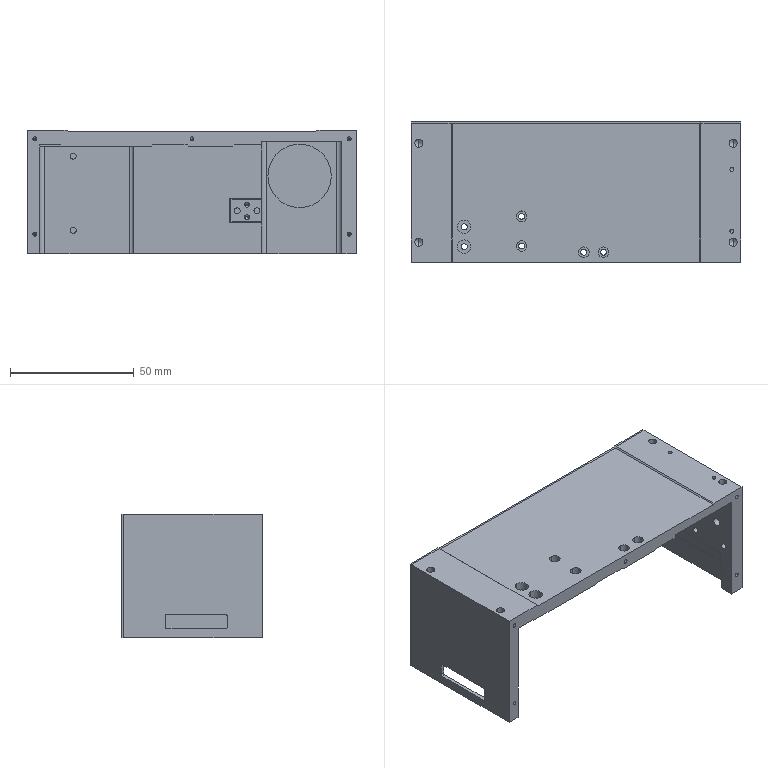NC program | NX | posted with a generic post | part box 133 x 56.74 x 50 mm
Lines 302 to 1465 of 22463:
(CAVITY_MILL , TOOL : D10)
N584 T10 M6
N586 G54
N588 G17 G0 G90 X4.555 Y-36.169 B0. C0. S9500 M3
N590 G43 Z30. H10
N592 Z1.005
N594 G94 G1 Z-0.495 F1000.
N596 X0.513 Y-29.169
N598 G3 X-0.353 Y-28.669 R1.
N600 G1 Y-7.669
N602 X37.695 F3000.
N604 G2 X38.9 Y-5.314 R26.1
N606 G1 Y-3.47
N608 X30.655
N610 G2 X23.5 Y-4.47 R26.1
N612 G1 X-28.25
N614 G2 X-38.4 Y-2.416 R26.1
N616 G1 Y-7.669
N618 X-0.353
N620 Y-14.669
N622 X42.762
N624 G2 X45.9 Y-7.35 R19.1
N626 G1 Y3.53
N628 X29.599
N630 G2 X23.5 Y2.53 R19.1
N632 G1 X-28.25
N634 G2 X-38.526 Y5.53 R19.1
N636 G1 X-45.4
N638 Y-10.674
N640 G2 X-43.021 Y-14.669 R19.1
N642 G1 X-0.353
N644 Y-21.669
N646 X49.4
N648 Y-18.37
N650 G2 X52.9 Y-9.858 R12.1
N652 G1 Y10.53
N654 X28.317
N656 G2 X23.5 Y9.53 R12.1
N658 G1 X-28.25
N660 G2 X-36.225 Y12.53 R12.1
N662 G1 X-49.527
N664 G2 X-52.4 Y8.641 R12.1
N666 G1 Y-13.381
N668 G2 X-48.42 Y-21.669 R12.1
N670 G1 X-0.353
N672 Y-28.669
N674 X55.007
N676 G3 X55.1 Y-29.506 R6.5
N678 G1 Y-33.169
N680 X56.5
N682 Y-29.375
N684 G2 X56.4 Y-28.37 R5.1
N686 G1 Y-18.37
N688 G2 X59.9 Y-13.527 R5.1
N690 G1 Y14.787
N692 G2 X56.852 Y17.53 R5.1
N694 G1 X26.533
N696 G2 X23.5 Y16.53 R5.1
N698 G1 X-28.25
N700 G2 X-32.898 Y19.53 R5.1
N702 G1 X-55.4
N704 Y17.395
N706 X-55.405 Y17.396
N708 G2 X-59.4 Y12.65 R5.1
N710 G1 Y-17.39
N712 G2 X-55.4 Y-22.37 R5.1
N714 G1 Y-28.37
N716 G2 X-55.5 Y-29.375 R5.1
N718 G1 Y-33.169
N720 X-54.1
N722 Y-29.506
N724 G3 X-54.007 Y-28.669 R6.5
N726 G1 X-0.353
N728 G2 X0.513 Y-29.169 R1.
N730 G1 X4.555 Y-36.169
N732 Z1.005
N734 G0 Z0.511
N736 G1 Z-0.989 F1000.
N738 X0.513 Y-29.169
N740 G3 X-0.353 Y-28.669 R1.
N742 G1 Y-7.669
N744 X37.695 F3000.
N746 G2 X38.9 Y-5.314 R26.1
N748 G1 Y-3.47
N750 X30.655
N752 G2 X23.5 Y-4.47 R26.1
N754 G1 X-28.25
N756 G2 X-38.4 Y-2.416 R26.1
N758 G1 Y-7.669
N760 X-0.353
N762 Y-14.669
N764 X42.762
N766 G2 X45.9 Y-7.35 R19.1
N768 G1 Y3.53
N770 X29.599
N772 G2 X23.5 Y2.53 R19.1
N774 G1 X-28.25
N776 G2 X-38.526 Y5.53 R19.1
N778 G1 X-45.4
N780 Y-10.674
N782 G2 X-43.021 Y-14.669 R19.1
N784 G1 X-0.353
N786 Y-21.669
N788 X49.4
N790 Y-18.369
N792 G2 X52.9 Y-9.858 R12.1
N794 G1 Y10.53
N796 X28.317
N798 G2 X23.5 Y9.53 R12.1
N800 G1 X-28.25
N802 G2 X-36.225 Y12.53 R12.1
N804 G1 X-49.527
N806 G2 X-52.4 Y8.641 R12.1
N808 G1 Y-13.381
N810 G2 X-48.42 Y-21.669 R12.1
N812 G1 X-0.353
N814 Y-28.669
N816 X55.007
N818 G3 X55.1 Y-29.506 R6.5
N820 G1 Y-33.169
N822 X56.5
N824 Y-29.375
N826 G2 X56.4 Y-28.37 R5.1
N828 G1 Y-21.669
N830 Y-18.369
N832 G2 X59.9 Y-13.527 R5.1
N834 G1 Y14.787
N836 G2 X56.852 Y17.53 R5.1
N838 G1 X26.533
N840 G2 X23.5 Y16.53 R5.1
N842 G1 X-28.25
N844 G2 X-32.898 Y19.53 R5.1
N846 G1 X-55.4
N848 Y17.395
N850 X-55.405 Y17.396
N852 G2 X-59.4 Y12.65 R5.1
N854 G1 Y-17.39
N856 G2 X-55.4 Y-22.37 R5.1
N858 G1 Y-28.37
N860 G2 X-55.5 Y-29.375 R5.1
N862 G1 Y-33.169
N864 X-54.1
N866 Y-29.506
N868 G3 X-54.007 Y-28.669 R6.5
N870 G1 X-0.353
N872 G2 X0.513 Y-29.169 R1.
N874 G1 X4.555 Y-36.169
N876 Z0.511
N878 G0 Z0.016
N880 G1 Z-1.484 F1000.
N882 X0.513 Y-29.169
N884 G3 X-0.353 Y-28.669 R1.
N886 G1 Y-7.669
N888 X37.695 F3000.
N890 G2 X38.9 Y-5.314 R26.1
N892 G1 Y-3.47
N894 X30.655
N896 G2 X23.5 Y-4.47 R26.1
N898 G1 X-28.25
N900 G2 X-38.4 Y-2.416 R26.1
N902 G1 Y-7.669
N904 X-0.353
N906 Y-14.669
N908 X42.762
N910 G2 X45.9 Y-7.35 R19.1
N912 G1 Y3.53
N914 X29.599
N916 G2 X23.5 Y2.53 R19.1
N918 G1 X-28.25
N920 G2 X-38.526 Y5.53 R19.1
N922 G1 X-45.4
N924 Y-10.674
N926 G2 X-43.021 Y-14.669 R19.1
N928 G1 X-0.353
N930 Y-21.669
N932 X49.4
N934 Y-18.37
N936 G2 X52.9 Y-9.858 R12.1
N938 G1 Y10.53
N940 X28.317
N942 G2 X23.5 Y9.53 R12.1
N944 G1 X-28.25
N946 G2 X-36.225 Y12.53 R12.1
N948 G1 X-49.527
N950 G2 X-52.4 Y8.641 R12.1
N952 G1 Y-13.381
N954 G2 X-48.42 Y-21.669 R12.1
N956 G1 X-0.353
N958 Y-28.669
N960 X55.007
N962 G3 X55.1 Y-29.506 R6.5
N964 G1 Y-33.169
N966 X56.5
N968 Y-29.375
N970 G2 X56.4 Y-28.37 R5.1
N972 G1 Y-18.37
N974 G2 X59.9 Y-13.527 R5.1
N976 G1 Y14.787
N978 G2 X56.852 Y17.53 R5.1
N980 G1 X26.533
N982 G2 X23.5 Y16.53 R5.1
N984 G1 X-28.25
N986 G2 X-32.898 Y19.53 R5.1
N988 G1 X-55.4
N990 Y17.395
N992 X-55.405 Y17.396
N994 G2 X-59.4 Y12.65 R5.1
N996 G1 Y-17.39
N998 G2 X-55.4 Y-22.37 R5.1
N1000 G1 Y-28.37
N1002 G2 X-55.5 Y-29.375 R5.1
N1004 G1 Y-33.169
N1006 X-54.1
N1008 Y-29.506
N1010 G3 X-54.007 Y-28.669 R6.5
N1012 G1 X-0.353
N1014 G2 X0.513 Y-29.169 R1.
N1016 G1 X4.555 Y-36.169
N1018 Z0.016
N1020 G0 Z-0.479
N1022 G1 Z-1.979 F1000.
N1024 X0.513 Y-29.169
N1026 G3 X-0.353 Y-28.669 R1.
N1028 G1 Y-7.669
N1030 X37.695 F3000.
N1032 G2 X38.9 Y-5.314 R26.1
N1034 G1 Y-3.47
N1036 X30.655
N1038 G2 X23.5 Y-4.47 R26.1
N1040 G1 X-28.25
N1042 G2 X-38.4 Y-2.416 R26.1
N1044 G1 Y-7.669
N1046 X-0.353
N1048 Y-14.669
N1050 X42.762
N1052 G2 X45.9 Y-7.35 R19.1
N1054 G1 Y3.53
N1056 X29.599
N1058 G2 X23.5 Y2.53 R19.1
N1060 G1 X-28.25
N1062 G2 X-38.526 Y5.53 R19.1
N1064 G1 X-45.4
N1066 Y-10.674
N1068 G2 X-43.021 Y-14.669 R19.1
N1070 G1 X-0.353
N1072 Y-21.669
N1074 X49.4
N1076 Y-18.37
N1078 G2 X52.9 Y-9.858 R12.1
N1080 G1 Y10.53
N1082 X28.317
N1084 G2 X23.5 Y9.53 R12.1
N1086 G1 X-28.25
N1088 G2 X-36.225 Y12.53 R12.1
N1090 G1 X-49.527
N1092 G2 X-52.4 Y8.641 R12.1
N1094 G1 Y-13.381
N1096 G2 X-48.42 Y-21.669 R12.1
N1098 G1 X-0.353
N1100 Y-28.669
N1102 X55.007
N1104 G3 X55.1 Y-29.506 R6.5
N1106 G1 Y-33.169
N1108 X56.5
N1110 Y-29.375
N1112 G2 X56.4 Y-28.37 R5.1
N1114 G1 Y-18.37
N1116 G2 X59.9 Y-13.527 R5.1
N1118 G1 Y14.787
N1120 G2 X56.852 Y17.53 R5.1
N1122 G1 X26.533
N1124 G2 X23.5 Y16.53 R5.1
N1126 G1 X-28.25
N1128 G2 X-32.898 Y19.53 R5.1
N1130 G1 X-55.4
N1132 Y17.395
N1134 X-55.405 Y17.396
N1136 G2 X-59.4 Y12.65 R5.1
N1138 G1 Y-17.39
N1140 G2 X-55.4 Y-22.37 R5.1
N1142 G1 Y-28.37
N1144 G2 X-55.5 Y-29.375 R5.1
N1146 G1 Y-33.169
N1148 X-54.1
N1150 Y-29.506
N1152 G3 X-54.007 Y-28.669 R6.5
N1154 G1 X-0.353
N1156 G2 X0.513 Y-29.169 R1.
N1158 G1 X4.555 Y-36.169
N1160 Z-0.479
N1162 G0 Z-0.974
N1164 G1 Z-2.474 F1000.
N1166 X0.513 Y-29.169
N1168 G3 X-0.353 Y-28.669 R1.
N1170 G1 Y-7.669
N1172 X37.695 F3000.
N1174 G2 X38.9 Y-5.314 R26.1
N1176 G1 Y-3.47
N1178 X30.655
N1180 G2 X23.5 Y-4.47 R26.1
N1182 G1 X-28.25
N1184 G2 X-38.4 Y-2.416 R26.1
N1186 G1 Y-7.669
N1188 X-0.353
N1190 Y-14.669
N1192 X42.762
N1194 G2 X45.9 Y-7.35 R19.1
N1196 G1 Y3.53
N1198 X29.599
N1200 G2 X23.5 Y2.53 R19.1
N1202 G1 X-28.25
N1204 G2 X-38.526 Y5.53 R19.1
N1206 G1 X-45.4
N1208 Y-10.674
N1210 G2 X-43.021 Y-14.669 R19.1
N1212 G1 X-0.353
N1214 Y-21.669
N1216 X49.4
N1218 Y-18.37
N1220 G2 X52.9 Y-9.858 R12.1
N1222 G1 Y10.53
N1224 X28.317
N1226 G2 X23.5 Y9.53 R12.1
N1228 G1 X-28.25
N1230 G2 X-36.225 Y12.53 R12.1
N1232 G1 X-49.527
N1234 G2 X-52.4 Y8.641 R12.1
N1236 G1 Y-13.381
N1238 G2 X-48.42 Y-21.669 R12.1
N1240 G1 X-0.353
N1242 Y-28.669
N1244 X55.007
N1246 G3 X55.1 Y-29.506 R6.5
N1248 G1 Y-33.169
N1250 X56.5
N1252 Y-29.375
N1254 G2 X56.4 Y-28.37 R5.1
N1256 G1 Y-18.37
N1258 G2 X59.9 Y-13.527 R5.1
N1260 G1 Y14.787
N1262 G2 X56.852 Y17.53 R5.1
N1264 G1 X26.533
N1266 G2 X23.5 Y16.53 R5.1
N1268 G1 X-28.25
N1270 G2 X-32.898 Y19.53 R5.1
N1272 G1 X-55.4
N1274 Y17.395
N1276 X-55.405 Y17.396
N1278 G2 X-59.4 Y12.65 R5.1
N1280 G1 Y-17.39
N1282 G2 X-55.4 Y-22.37 R5.1
N1284 G1 Y-28.37
N1286 G2 X-55.5 Y-29.375 R5.1
N1288 G1 Y-33.169
N1290 X-54.1
N1292 Y-29.506
N1294 G3 X-54.007 Y-28.669 R6.5
N1296 G1 X-0.353
N1298 G2 X0.513 Y-29.169 R1.
N1300 G1 X4.555 Y-36.169
N1302 Z-0.974
N1304 G0 Z-1.468
N1306 G1 Z-2.968 F1000.
N1308 X0.513 Y-29.169
N1310 G3 X-0.353 Y-28.669 R1.
N1312 G1 Y-7.669
N1314 X37.695 F3000.
N1316 G2 X38.9 Y-5.314 R26.1
N1318 G1 Y-3.47
N1320 X30.655
N1322 G2 X23.5 Y-4.47 R26.1
N1324 G1 X-28.25
N1326 G2 X-38.4 Y-2.416 R26.1
N1328 G1 Y-7.669
N1330 X-0.353
N1332 Y-14.669
N1334 X42.762
N1336 G2 X45.9 Y-7.35 R19.1
N1338 G1 Y3.53
N1340 X29.599
N1342 G2 X23.5 Y2.53 R19.1
N1344 G1 X-28.25
N1346 G2 X-38.526 Y5.53 R19.1
N1348 G1 X-45.4
N1350 Y-10.674
N1352 G2 X-43.021 Y-14.669 R19.1
N1354 G1 X-0.353
N1356 Y-21.669
N1358 X49.4
N1360 Y-18.37
N1362 G2 X52.9 Y-9.858 R12.1
N1364 G1 Y10.53
N1366 X28.317
N1368 G2 X23.5 Y9.53 R12.1
N1370 G1 X-28.25
N1372 G2 X-36.225 Y12.53 R12.1
N1374 G1 X-49.527
N1376 G2 X-52.4 Y8.641 R12.1
N1378 G1 Y-13.381
N1380 G2 X-48.42 Y-21.669 R12.1
N1382 G1 X-0.353
N1384 Y-28.669
N1386 X55.007
N1388 G3 X55.1 Y-29.506 R6.5
N1390 G1 Y-33.169
N1392 X56.5
N1394 Y-29.375
N1396 G2 X56.4 Y-28.37 R5.1
N1398 G1 Y-18.37
N1400 G2 X59.9 Y-13.527 R5.1
N1402 G1 Y14.787
N1404 G2 X56.852 Y17.53 R5.1
N1406 G1 X26.533
N1408 G2 X23.5 Y16.53 R5.1
N1410 G1 X-28.25
N1412 G2 X-32.898 Y19.53 R5.1
N1414 G1 X-55.4
N1416 Y17.395
N1418 X-55.405 Y17.396
N1420 G2 X-59.4 Y12.65 R5.1
N1422 G1 Y-17.39
N1424 G2 X-55.4 Y-22.37 R5.1
N1426 G1 Y-28.37
N1428 G2 X-55.5 Y-29.375 R5.1
N1430 G1 Y-33.169
N1432 X-54.1
N1434 Y-29.506
N1436 G3 X-54.007 Y-28.669 R6.5
N1438 G1 X-0.353
N1440 G2 X0.513 Y-29.169 R1.
N1442 G1 X4.555 Y-36.169
N1444 Z-1.468
N1446 G0 Z-1.963
N1448 G1 Z-3.463 F1000.
N1450 X0.513 Y-29.169
N1452 G3 X-0.353 Y-28.669 R1.
N1454 G1 Y-7.669
N1456 X37.695 F3000.
N1458 G2 X38.9 Y-5.314 R26.1
N1460 G1 Y-3.47
N1462 X30.655
N1464 G2 X23.5 Y-4.47 R26.1
N1466 G1 X-28.25
N1468 G2 X-38.4 Y-2.416 R26.1
N1470 G1 Y-7.669
N1472 X-0.353
N1474 Y-14.669
N1476 X42.762
N1478 G2 X45.9 Y-7.35 R19.1
N1480 G1 Y3.53
N1482 X29.599
N1484 G2 X23.5 Y2.53 R19.1
N1486 G1 X-28.25
N1488 G2 X-38.526 Y5.53 R19.1
N1490 G1 X-45.4
N1492 Y-10.674
N1494 G2 X-43.021 Y-14.669 R19.1
N1496 G1 X-0.353
N1498 Y-21.669
N1500 X49.4
N1502 Y-18.37
N1504 G2 X52.9 Y-9.858 R12.1
N1506 G1 Y10.53
N1508 X28.317
N1510 G2 X23.5 Y9.53 R12.1
N1512 G1 X-28.25
N1514 G2 X-36.225 Y12.53 R12.1
N1516 G1 X-49.527
N1518 G2 X-52.4 Y8.641 R12.1
N1520 G1 Y-13.381
N1522 G2 X-48.42 Y-21.669 R12.1
N1524 G1 X-0.353
N1526 Y-28.669
N1528 X55.007
N1530 G3 X55.1 Y-29.506 R6.5
N1532 G1 Y-33.169
N1534 X56.5
N1536 Y-29.375
N1538 G2 X56.4 Y-28.37 R5.1
N1540 G1 Y-18.37
N1542 G2 X59.9 Y-13.527 R5.1
N1544 G1 Y14.787
N1546 G2 X56.852 Y17.53 R5.1
N1548 G1 X26.533
N1550 G2 X23.5 Y16.53 R5.1
N1552 G1 X-28.25
N1554 G2 X-32.898 Y19.53 R5.1
N1556 G1 X-55.4
N1558 Y17.395
N1560 X-55.405 Y17.396
N1562 G2 X-59.4 Y12.65 R5.1
N1564 G1 Y-17.39
N1566 G2 X-55.4 Y-22.37 R5.1
N1568 G1 Y-28.37
N1570 G2 X-55.5 Y-29.375 R5.1
N1572 G1 Y-33.169
N1574 X-54.1
N1576 Y-29.506
N1578 G3 X-54.007 Y-28.669 R6.5
N1580 G1 X-0.353
N1582 G2 X0.513 Y-29.169 R1.
N1584 G1 X4.555 Y-36.169
N1586 Z-1.963
N1588 G0 Z-2.458
N1590 G1 Z-3.958 F1000.
N1592 X0.513 Y-29.169
N1594 G3 X-0.353 Y-28.669 R1.
N1596 G1 Y-7.669
N1598 X37.695 F3000.
N1600 G2 X38.9 Y-5.314 R26.1
N1602 G1 Y-3.47
N1604 X30.655
N1606 G2 X23.5 Y-4.47 R26.1
N1608 G1 X-28.25
N1610 G2 X-38.4 Y-2.416 R26.1
N1612 G1 Y-7.669
N1614 X-0.353
N1616 Y-14.669
N1618 X42.762
N1620 G2 X45.9 Y-7.35 R19.1
N1622 G1 Y3.53
N1624 X29.599
N1626 G2 X23.5 Y2.53 R19.1
N1628 G1 X-28.25
N1630 G2 X-38.526 Y5.53 R19.1
N1632 G1 X-45.4
N1634 Y-10.674
N1636 G2 X-43.021 Y-14.669 R19.1
N1638 G1 X-0.353
N1640 Y-21.669
N1642 X49.4
N1644 Y-18.37
N1646 G2 X52.9 Y-9.858 R12.1
N1648 G1 Y10.53
N1650 X28.317
N1652 G2 X23.5 Y9.53 R12.1
N1654 G1 X-28.25
N1656 G2 X-36.225 Y12.53 R12.1
N1658 G1 X-49.527
N1660 G2 X-52.4 Y8.641 R12.1
N1662 G1 Y-13.381
N1664 G2 X-48.42 Y-21.669 R12.1
N1666 G1 X-0.353
N1668 Y-28.669
N1670 X55.007
N1672 G3 X55.1 Y-29.506 R6.5
N1674 G1 Y-33.169
N1676 X56.5
N1678 Y-29.375
N1680 G2 X56.4 Y-28.37 R5.1
N1682 G1 Y-18.37
N1684 G2 X59.9 Y-13.527 R5.1
N1686 G1 Y14.787
N1688 G2 X56.852 Y17.53 R5.1
N1690 G1 X26.533
N1692 G2 X23.5 Y16.53 R5.1
N1694 G1 X-28.25
N1696 G2 X-32.898 Y19.53 R5.1
N1698 G1 X-55.4
N1700 Y17.395
N1702 X-55.405 Y17.396
N1704 G2 X-59.4 Y12.65 R5.1
N1706 G1 Y-17.39
N1708 G2 X-55.4 Y-22.37 R5.1
N1710 G1 Y-28.37
N1712 G2 X-55.5 Y-29.375 R5.1
N1714 G1 Y-33.169
N1716 X-54.1
N1718 Y-29.506
N1720 G3 X-54.007 Y-28.669 R6.5
N1722 G1 X-0.353
N1724 G2 X0.513 Y-29.169 R1.
N1726 G1 X4.555 Y-36.169
N1728 Z-2.458
N1730 G0 Z-2.953
N1732 G1 Z-4.453 F1000.
N1734 X0.513 Y-29.169
N1736 G3 X-0.353 Y-28.669 R1.
N1738 G1 Y-7.669
N1740 X37.695 F3000.
N1742 G2 X38.9 Y-5.314 R26.1
N1744 G1 Y-3.47
N1746 X30.655
N1748 G2 X23.5 Y-4.47 R26.1
N1750 G1 X-28.25
N1752 G2 X-38.4 Y-2.416 R26.1
N1754 G1 Y-7.669
N1756 X-0.353
N1758 Y-14.669
N1760 X42.762
N1762 G2 X45.9 Y-7.35 R19.1
N1764 G1 Y3.53
N1766 X29.599
N1768 G2 X23.5 Y2.53 R19.1
N1770 G1 X-28.25
N1772 G2 X-38.526 Y5.53 R19.1
N1774 G1 X-45.4
N1776 Y-10.674
N1778 G2 X-43.021 Y-14.669 R19.1
N1780 G1 X-0.353
N1782 Y-21.669
N1784 X49.4
N1786 Y-18.37
N1788 G2 X52.9 Y-9.858 R12.1
N1790 G1 Y10.53
N1792 X28.317
N1794 G2 X23.5 Y9.53 R12.1
N1796 G1 X-28.25
N1798 G2 X-36.225 Y12.53 R12.1
N1800 G1 X-49.527
N1802 G2 X-52.4 Y8.641 R12.1
N1804 G1 Y-13.381
N1806 G2 X-48.42 Y-21.669 R12.1
N1808 G1 X-0.353
N1810 Y-28.669
N1812 X55.007
N1814 G3 X55.1 Y-29.506 R6.5
N1816 G1 Y-33.169
N1818 X56.5
N1820 Y-29.375
N1822 G2 X56.4 Y-28.37 R5.1
N1824 G1 Y-18.37
N1826 G2 X59.9 Y-13.527 R5.1
N1828 G1 Y14.787
N1830 G2 X56.852 Y17.53 R5.1
N1832 G1 X26.533
N1834 G2 X23.5 Y16.53 R5.1
N1836 G1 X-28.25
N1838 G2 X-32.898 Y19.53 R5.1
N1840 G1 X-55.4
N1842 X-55.405 Y17.396
N1844 G2 X-59.4 Y12.65 R5.1
N1846 G1 Y-17.39
N1848 G2 X-55.4 Y-22.37 R5.1
N1850 G1 Y-28.37
N1852 G2 X-55.5 Y-29.375 R5.1
N1854 G1 Y-33.169
N1856 X-54.1
N1858 Y-29.506
N1860 G3 X-54.007 Y-28.669 R6.5
N1862 G1 X-0.353
N1864 G2 X0.513 Y-29.169 R1.
N1866 G1 X4.555 Y-36.169
N1868 Z-2.953
N1870 G0 Z-3.447
N1872 G1 Z-4.947 F1000.
N1874 X0.513 Y-29.169
N1876 G3 X-0.353 Y-28.669 R1.
N1878 G1 Y-7.669
N1880 X37.695 F3000.
N1882 G2 X38.9 Y-5.314 R26.1
N1884 G1 Y-3.47
N1886 X30.655
N1888 G2 X23.5 Y-4.47 R26.1
N1890 G1 X-28.25
N1892 G2 X-38.4 Y-2.416 R26.1
N1894 G1 Y-7.669
N1896 X-0.353
N1898 Y-14.669
N1900 X42.762
N1902 G2 X45.9 Y-7.35 R19.1
N1904 G1 Y3.53
N1906 X29.599
N1908 G2 X23.5 Y2.53 R19.1
N1910 G1 X-28.25
N1912 G2 X-38.526 Y5.53 R19.1
N1914 G1 X-45.4
N1916 Y-10.674
N1918 G2 X-43.021 Y-14.669 R19.1
N1920 G1 X-0.353
N1922 Y-21.669
N1924 X49.4
N1926 Y-18.37
N1928 G2 X52.9 Y-9.858 R12.1
N1930 G1 Y10.53
N1932 X28.317
N1934 G2 X23.5 Y9.53 R12.1
N1936 G1 X-28.25
N1938 G2 X-36.225 Y12.53 R12.1
N1940 G1 X-49.527
N1942 G2 X-52.4 Y8.641 R12.1
N1944 G1 Y-13.381
N1946 G2 X-48.42 Y-21.669 R12.1
N1948 G1 X-0.353
N1950 Y-28.669
N1952 X55.007
N1954 G3 X55.1 Y-29.506 R6.5
N1956 G1 Y-33.169
N1958 X56.5
N1960 Y-29.375
N1962 G2 X56.4 Y-28.37 R5.1
N1964 G1 Y-18.37
N1966 G2 X59.9 Y-13.527 R5.1
N1968 G1 Y14.787
N1970 G2 X56.852 Y17.53 R5.1
N1972 G1 X26.533
N1974 G2 X23.5 Y16.53 R5.1
N1976 G1 X-28.25
N1978 G2 X-32.898 Y19.53 R5.1
N1980 G1 X-55.4
N1982 Y17.395
N1984 X-55.405 Y17.396
N1986 G2 X-59.4 Y12.65 R5.1
N1988 G1 Y-17.39
N1990 G2 X-55.4 Y-22.37 R5.1
N1992 G1 Y-28.37
N1994 G2 X-55.5 Y-29.375 R5.1
N1996 G1 Y-33.169
N1998 X-54.1
N2000 Y-29.506
N2002 G3 X-54.007 Y-28.669 R6.5
N2004 G1 X-0.353
N2006 G2 X0.513 Y-29.169 R1.
N2008 G1 X4.555 Y-36.169
N2010 Z-3.447
N2012 G0 Z-3.942
N2014 G1 Z-5.442 F1000.
N2016 X0.513 Y-29.169
N2018 G3 X-0.353 Y-28.669 R1.
N2020 G1 Y-7.669
N2022 X37.695 F3000.
N2024 G2 X38.9 Y-5.314 R26.1
N2026 G1 Y-3.47
N2028 X30.655
N2030 G2 X23.5 Y-4.47 R26.1
N2032 G1 X-28.25
N2034 G2 X-38.4 Y-2.416 R26.1
N2036 G1 Y-7.669
N2038 X-0.353
N2040 Y-14.669
N2042 X42.762
N2044 G2 X45.9 Y-7.35 R19.1
N2046 G1 Y3.53
N2048 X29.599
N2050 G2 X23.5 Y2.53 R19.1
N2052 G1 X-28.25
N2054 G2 X-38.526 Y5.53 R19.1
N2056 G1 X-45.4
N2058 Y-10.674
N2060 G2 X-43.021 Y-14.669 R19.1
N2062 G1 X-0.353
N2064 Y-21.669
N2066 X49.4
N2068 Y-18.37
N2070 G2 X52.9 Y-9.858 R12.1
N2072 G1 Y10.53
N2074 X28.317
N2076 G2 X23.5 Y9.53 R12.1
N2078 G1 X-28.25
N2080 G2 X-36.225 Y12.53 R12.1
N2082 G1 X-49.527
N2084 G2 X-52.4 Y8.641 R12.1
N2086 G1 Y-13.381
N2088 G2 X-48.42 Y-21.669 R12.1
N2090 G1 X-0.353
N2092 Y-28.669
N2094 X55.007
N2096 G3 X55.1 Y-29.506 R6.5
N2098 G1 Y-33.169
N2100 X56.5
N2102 Y-29.375
N2104 G2 X56.4 Y-28.37 R5.1
N2106 G1 Y-18.37
N2108 G2 X59.9 Y-13.527 R5.1
N2110 G1 Y14.787
N2112 G2 X56.852 Y17.53 R5.1
N2114 G1 X26.533
N2116 G2 X23.5 Y16.53 R5.1
N2118 G1 X-28.25
N2120 G2 X-32.898 Y19.53 R5.1
N2122 G1 X-55.4
N2124 Y17.395
N2126 X-55.405 Y17.396
N2128 G2 X-59.4 Y12.65 R5.1
N2130 G1 Y-17.39
N2132 G2 X-55.4 Y-22.37 R5.1
N2134 G1 Y-28.37
N2136 G2 X-55.5 Y-29.375 R5.1
N2138 G1 Y-33.169
N2140 X-54.1
N2142 Y-29.506
N2144 G3 X-54.007 Y-28.669 R6.5
N2146 G1 X-0.353
N2148 G2 X0.513 Y-29.169 R1.
N2150 G1 X4.555 Y-36.169
N2152 Z-3.942
N2154 G0 Z-4.437
N2156 G1 Z-5.937 F1000.
N2158 X0.513 Y-29.169
N2160 G3 X-0.353 Y-28.669 R1.
N2162 G1 Y-7.669
N2164 X37.695 F3000.
N2166 G2 X38.9 Y-5.314 R26.1
N2168 G1 Y-3.47
N2170 X30.655
N2172 G2 X23.5 Y-4.47 R26.1
N2174 G1 X-28.25
N2176 G2 X-38.4 Y-2.416 R26.1
N2178 G1 Y-7.669
N2180 X-0.353
N2182 Y-14.669
N2184 X42.762
N2186 G2 X45.9 Y-7.35 R19.1
N2188 G1 Y3.53
N2190 X29.599
N2192 G2 X23.5 Y2.53 R19.1
N2194 G1 X-28.25
N2196 G2 X-38.526 Y5.53 R19.1
N2198 G1 X-45.4
N2200 Y-10.674
N2202 G2 X-43.021 Y-14.669 R19.1
N2204 G1 X-0.353
N2206 Y-21.669
N2208 X49.4
N2210 Y-18.37
N2212 G2 X52.9 Y-9.858 R12.1
N2214 G1 Y10.53
N2216 X28.317
N2218 G2 X23.5 Y9.53 R12.1
N2220 G1 X-28.25
N2222 G2 X-36.225 Y12.53 R12.1
N2224 G1 X-49.527
N2226 G2 X-52.4 Y8.641 R12.1
N2228 G1 Y-13.381
N2230 G2 X-48.42 Y-21.669 R12.1
N2232 G1 X-0.353
N2234 Y-28.669
N2236 X55.007
N2238 G3 X55.1 Y-29.506 R6.5
N2240 G1 Y-33.169
N2242 X56.5
N2244 Y-29.375
N2246 G2 X56.4 Y-28.37 R5.1
N2248 G1 Y-18.37
N2250 G2 X59.9 Y-13.527 R5.1
N2252 G1 Y14.787
N2254 G2 X56.852 Y17.53 R5.1
N2256 G1 X26.533
N2258 G2 X23.5 Y16.53 R5.1
N2260 G1 X-28.25
N2262 G2 X-32.898 Y19.53 R5.1
N2264 G1 X-55.4
N2266 Y17.395
N2268 X-55.405 Y17.396
N2270 G2 X-59.4 Y12.65 R5.1
N2272 G1 Y-17.39
N2274 G2 X-55.4 Y-22.37 R5.1
N2276 G1 Y-28.37
N2278 G2 X-55.5 Y-29.375 R5.1
N2280 G1 Y-33.169
N2282 X-54.1
N2284 Y-29.506
N2286 G3 X-54.007 Y-28.669 R6.5
N2288 G1 X-0.353
N2290 G2 X0.513 Y-29.169 R1.
N2292 G1 X4.555 Y-36.169
N2294 Z-4.437
N2296 G0 Z-4.932
N2298 G1 Z-6.432 F1000.
N2300 X0.513 Y-29.169
N2302 G3 X-0.353 Y-28.669 R1.
N2304 G1 Y-7.669
N2306 X37.695 F3000.
N2308 G2 X38.9 Y-5.314 R26.1
N2310 G1 Y-3.47
N2312 X30.655
N2314 G2 X23.5 Y-4.47 R26.1
N2316 G1 X-28.25
N2318 G2 X-38.4 Y-2.416 R26.1
N2320 G1 Y-7.669
N2322 X-0.353
N2324 Y-14.669
N2326 X42.762
N2328 G2 X45.9 Y-7.35 R19.1
N2330 G1 Y3.53
N2332 X29.599
N2334 G2 X23.5 Y2.53 R19.1
N2336 G1 X-28.25
N2338 G2 X-38.526 Y5.53 R19.1
N2340 G1 X-45.4
N2342 Y-10.674
N2344 G2 X-43.021 Y-14.669 R19.1
N2346 G1 X-0.353
N2348 Y-21.669
N2350 X49.4
N2352 Y-18.37
N2354 G2 X52.9 Y-9.858 R12.1
N2356 G1 Y10.53
N2358 X28.317
N2360 G2 X23.5 Y9.53 R12.1
N2362 G1 X-28.25
N2364 G2 X-36.225 Y12.53 R12.1
N2366 G1 X-49.527
N2368 G2 X-52.4 Y8.641 R12.1
N2370 G1 Y-13.381
N2372 G2 X-48.42 Y-21.669 R12.1
N2374 G1 X-0.353
N2376 Y-28.669
N2378 X55.007
N2380 G3 X55.1 Y-29.506 R6.5
N2382 G1 Y-33.169
N2384 X56.5
N2386 Y-29.375
N2388 G2 X56.4 Y-28.37 R5.1
N2390 G1 Y-18.37
N2392 G2 X59.9 Y-13.527 R5.1
N2394 G1 Y14.787
N2396 G2 X56.852 Y17.53 R5.1
N2398 G1 X26.533
N2400 G2 X23.5 Y16.53 R5.1
N2402 G1 X-28.25
N2404 G2 X-32.898 Y19.53 R5.1
N2406 G1 X-55.4
N2408 X-55.405 Y17.396
N2410 G2 X-59.4 Y12.65 R5.1
N2412 G1 Y-17.39
N2414 G2 X-55.4 Y-22.37 R5.1
N2416 G1 Y-28.37
N2418 G2 X-55.5 Y-29.375 R5.1
N2420 G1 Y-33.169
N2422 X-54.1
N2424 Y-29.506
N2426 G3 X-54.007 Y-28.669 R6.5
N2428 G1 X-0.353
N2430 G2 X0.513 Y-29.169 R1.
N2432 G1 X4.555 Y-36.169
N2434 Z-4.932
N2436 G0 Z-5.426
N2438 G1 Z-6.926 F1000.
N2440 X0.513 Y-29.169
N2442 G3 X-0.353 Y-28.669 R1.
N2444 G1 Y-7.669
N2446 X37.695 F3000.
N2448 G2 X38.9 Y-5.314 R26.1
N2450 G1 Y-3.47
N2452 X30.655
N2454 G2 X23.5 Y-4.47 R26.1
N2456 G1 X-28.25
N2458 G2 X-38.4 Y-2.416 R26.1
N2460 G1 Y-7.669
N2462 X-0.353
N2464 Y-14.669
N2466 X42.762
N2468 G2 X45.9 Y-7.35 R19.1
N2470 G1 Y3.53
N2472 X29.599
N2474 G2 X23.5 Y2.53 R19.1
N2476 G1 X-28.25
N2478 G2 X-38.526 Y5.53 R19.1
N2480 G1 X-45.4
N2482 Y-10.674
N2484 G2 X-43.021 Y-14.669 R19.1
N2486 G1 X-0.353
N2488 Y-21.669
N2490 X49.4
N2492 Y-18.37
N2494 G2 X52.9 Y-9.858 R12.1
N2496 G1 Y10.53
N2498 X28.317
N2500 G2 X23.5 Y9.53 R12.1
N2502 G1 X-28.25
N2504 G2 X-36.225 Y12.53 R12.1
N2506 G1 X-49.527
N2508 G2 X-52.4 Y8.641 R12.1
N2510 G1 Y-13.381
N2512 G2 X-48.42 Y-21.669 R12.1
N2514 G1 X-0.353
N2516 Y-28.669
N2518 X55.007
N2520 G3 X55.1 Y-29.506 R6.5
N2522 G1 Y-33.169
N2524 X56.5
N2526 Y-29.375
N2528 G2 X56.4 Y-28.37 R5.1
N2530 G1 Y-18.37
N2532 G2 X59.9 Y-13.527 R5.1
N2534 G1 Y14.787
N2536 G2 X56.852 Y17.53 R5.1
N2538 G1 X26.533
N2540 G2 X23.5 Y16.53 R5.1
N2542 G1 X-28.25
N2544 G2 X-32.898 Y19.53 R5.1
N2546 G1 X-55.4
N2548 Y17.395
N2550 X-55.405 Y17.396
N2552 G2 X-59.4 Y12.65 R5.1
N2554 G1 Y-17.39
N2556 G2 X-55.4 Y-22.37 R5.1
N2558 G1 Y-28.37
N2560 G2 X-55.5 Y-29.375 R5.1
N2562 G1 Y-33.169
N2564 X-54.1
N2566 Y-29.506
N2568 G3 X-54.007 Y-28.669 R6.5
N2570 G1 X-0.353
N2572 G2 X0.513 Y-29.169 R1.
N2574 G1 X4.555 Y-36.169
N2576 Z-5.426
N2578 G0 Z-5.921
N2580 G1 Z-7.421 F1000.
N2582 X0.513 Y-29.169
N2584 G3 X-0.353 Y-28.669 R1.
N2586 G1 Y-7.669
N2588 X37.695 F3000.
N2590 G2 X38.9 Y-5.314 R26.1
N2592 G1 Y-3.47
N2594 X30.655
N2596 G2 X23.5 Y-4.47 R26.1
N2598 G1 X-28.25
N2600 G2 X-38.4 Y-2.416 R26.1
N2602 G1 Y-7.669
N2604 X-0.353
N2606 Y-14.669
N2608 X42.762
N2610 G2 X45.9 Y-7.35 R19.1
N2612 G1 Y3.53
N2614 X29.599
N2616 G2 X23.5 Y2.53 R19.1
N2618 G1 X-28.25
N2620 G2 X-38.526 Y5.53 R19.1
N2622 G1 X-45.4
N2624 Y-10.674
N2626 G2 X-43.021 Y-14.669 R19.1
N2628 G1 X-0.353
N2630 Y-21.669
N2632 X49.4
N2634 Y-18.37
N2636 G2 X52.9 Y-9.858 R12.1
N2638 G1 Y10.53
N2640 X28.317
N2642 G2 X23.5 Y9.53 R12.1
N2644 G1 X-28.25
N2646 G2 X-36.225 Y12.53 R12.1
N2648 G1 X-49.527
N2650 G2 X-52.4 Y8.641 R12.1
N2652 G1 Y-13.381
N2654 G2 X-48.42 Y-21.669 R12.1
N2656 G1 X-0.353
N2658 Y-28.669
N2660 X55.007
N2662 G3 X55.1 Y-29.506 R6.5
N2664 G1 Y-33.169
N2666 X56.5
N2668 Y-29.375
N2670 G2 X56.4 Y-28.37 R5.1
N2672 G1 Y-18.37
N2674 G2 X59.9 Y-13.527 R5.1
N2676 G1 Y14.787
N2678 G2 X56.852 Y17.53 R5.1
N2680 G1 X26.533
N2682 G2 X23.5 Y16.53 R5.1
N2684 G1 X-28.25
N2686 G2 X-32.898 Y19.53 R5.1
N2688 G1 X-55.4
N2690 Y17.395
N2692 X-55.405 Y17.396
N2694 G2 X-59.4 Y12.65 R5.1
N2696 G1 Y-17.39
N2698 G2 X-55.4 Y-22.37 R5.1
N2700 G1 Y-28.37
N2702 G2 X-55.5 Y-29.375 R5.1
N2704 G1 Y-33.169
N2706 X-54.1
N2708 Y-29.506
N2710 G3 X-54.007 Y-28.669 R6.5
N2712 G1 X-0.353
N2714 G2 X0.513 Y-29.169 R1.
N2716 G1 X4.555 Y-36.169
N2718 Z-5.921
N2720 G0 Z-6.416
N2722 G1 Z-7.916 F1000.
N2724 X0.513 Y-29.169
N2726 G3 X-0.353 Y-28.669 R1.
N2728 G1 Y-7.669
N2730 X37.695 F3000.
N2732 G2 X38.9 Y-5.314 R26.1
N2734 G1 Y-3.47
N2736 X30.655
N2738 G2 X23.5 Y-4.47 R26.1
N2740 G1 X-28.25
N2742 G2 X-38.4 Y-2.416 R26.1
N2744 G1 Y-7.669
N2746 X-0.353
N2748 Y-14.669
N2750 X42.762
N2752 G2 X45.9 Y-7.35 R19.1
N2754 G1 Y3.53
N2756 X29.599
N2758 G2 X23.5 Y2.53 R19.1
N2760 G1 X-28.25
N2762 G2 X-38.526 Y5.53 R19.1
N2764 G1 X-45.4
N2766 Y-10.674
N2768 G2 X-43.021 Y-14.669 R19.1
N2770 G1 X-0.353
N2772 Y-21.669
N2774 X49.4
N2776 Y-18.37
N2778 G2 X52.9 Y-9.858 R12.1
N2780 G1 Y10.53
N2782 X28.317
N2784 G2 X23.5 Y9.53 R12.1
N2786 G1 X-28.25
N2788 G2 X-36.225 Y12.53 R12.1
N2790 G1 X-49.527
N2792 G2 X-52.4 Y8.641 R12.1
N2794 G1 Y-13.381
N2796 G2 X-48.42 Y-21.669 R12.1
N2798 G1 X-0.353
N2800 Y-28.669
N2802 X55.007
N2804 G3 X55.1 Y-29.506 R6.5
N2806 G1 Y-33.169
N2808 X56.5
N2810 Y-29.375
N2812 G2 X56.4 Y-28.37 R5.1
N2814 G1 Y-18.37
N2816 G2 X59.9 Y-13.527 R5.1
N2818 G1 Y14.787
N2820 G2 X56.852 Y17.53 R5.1
N2822 G1 X26.533
N2824 G2 X23.5 Y16.53 R5.1
N2826 G1 X-28.25
N2828 G2 X-32.898 Y19.53 R5.1
N2830 G1 X-55.4
N2832 Y17.395
N2834 X-55.405 Y17.396
N2836 G2 X-59.4 Y12.65 R5.1
N2838 G1 Y-17.39
N2840 G2 X-55.4 Y-22.37 R5.1
N2842 G1 Y-28.37
N2844 G2 X-55.5 Y-29.375 R5.1
N2846 G1 Y-33.169
N2848 X-54.1
N2850 Y-29.506
N2852 G3 X-54.007 Y-28.669 R6.5
N2854 G1 X-0.353
N2856 G2 X0.513 Y-29.169 R1.
N2858 G1 X4.555 Y-36.169
N2860 Z-6.416
N2862 G0 Z-6.911
N2864 G1 Z-8.411 F1000.
N2866 X0.513 Y-29.169
N2868 G3 X-0.353 Y-28.669 R1.
N2870 G1 Y-7.669
N2872 X37.695 F3000.
N2874 G2 X38.9 Y-5.314 R26.1
N2876 G1 Y-3.47
N2878 X30.655
N2880 G2 X23.5 Y-4.47 R26.1
N2882 G1 X-28.25
N2884 G2 X-38.4 Y-2.416 R26.1
N2886 G1 Y-7.669
N2888 X-0.353
N2890 Y-14.669
N2892 X42.762
N2894 G2 X45.9 Y-7.35 R19.1
N2896 G1 Y3.53
N2898 X29.599
N2900 G2 X23.5 Y2.53 R19.1
N2902 G1 X-28.25
N2904 G2 X-38.526 Y5.53 R19.1